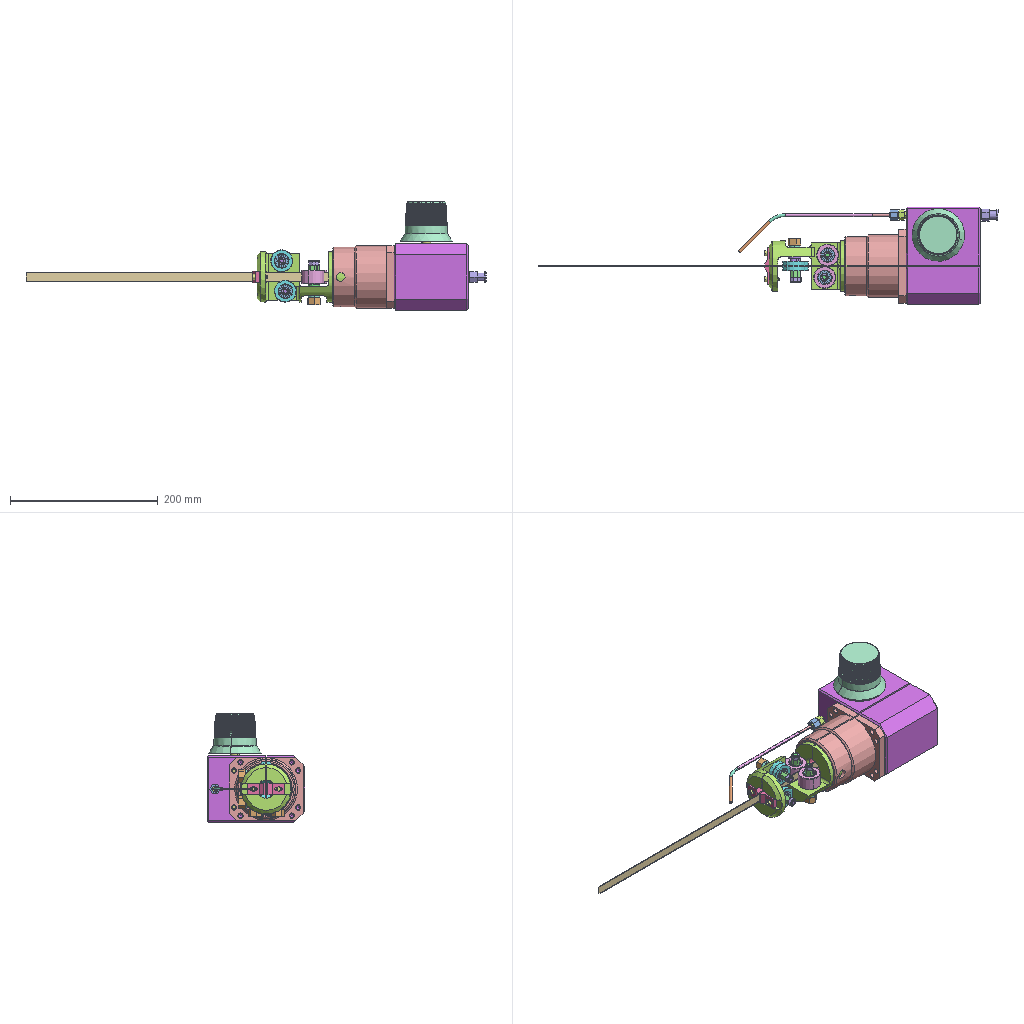Assembly | SolidWorks | 31 different items | 61 placed | box 622 x 132 x 147 mm
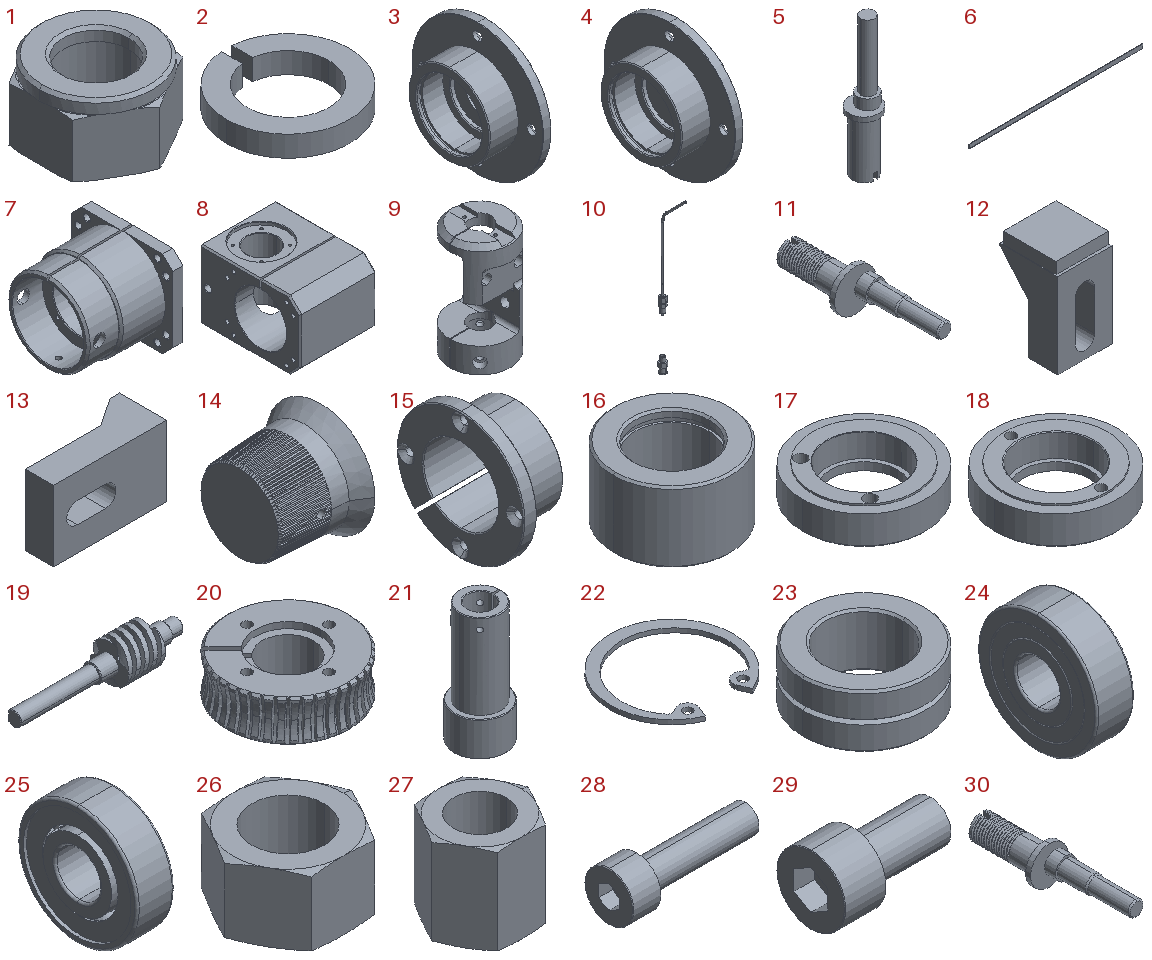Parts list (item | name | quantity | size | volume | features):
1 | - | x4 | 9.8 x 11.05 x 6 mm | 303.009 mm3 | features Cut 3, Boss 1, Chamfer 1, Extrusion 1, MoveFace 1
2 | - | x4 | 15.372 x 15.344 x 2.6 mm | 261.313 mm3 | features Extrusion 1
3 | - | x1 | 18 x 64.5 x 64.5 mm | 18239 mm3 | features CirPattern 2, ICE 2, Chamfer 1, HoleWzd 1, RevCut 1, Revolution 1
4 | - | x1 | 18 x 64.5 x 64.5 mm | 18637 mm3 | features CirPattern 2, Chamfer 1, HoleWzd 1, ICE 1, RevCut 1, Revolution 1
5 | - | x1 | 13 x 13 x 59.5 mm | 3175 mm3 | features ICE 5, Extrusion 1
6 | - | x1 | 503 x 0.6 x 13 mm | 3620 mm3 | features ICE 2, Extrusion 1
7 | - | x1 | 83.2 x 100 x 85 mm | 237929 mm3 | features ICE 5, Chamfer 4, MoveFace 4, MirrorPattern 3, CirPattern 1, DelFace 1, Fillet 1, HoleWzd 1, LockFeature 1, Revolution 1
8 | - | x1 | 100 x 132.3 x 90 mm | 668106 mm3 | features Chamfer 7, ICE 7, HoleWzd 5, DelFace 4, MoveFace 2, CirPattern 1, Extrusion 1, MirrorPattern 1
9 | - | x1 | 67.996 x 68 x 125 mm | 160312 mm3 | features ICE 17, Fillet 8, MoveFace 7, HoleWzd 3, Chamfer 2, DelFace 1, Extrusion 1, MirrorPattern 1
10 | - | x1 | 14 x 58.995 x 350.912 mm | 7220 mm3 | features ICE 8, MoveCopyBody 2, Chamfer 1, MirrorSolid 1, WeldMemberFeat 1, WeldmentFeature 1
11 | - | x2 | 17 x 59.6 x 17 mm | 3396 mm3 | features ICE 5, Chamfer 2, Extrusion 1, SweepThread 1
12 | - | x2 | 14 x 15 x 25 mm | 2645 mm3 | features ICE 4, Extrusion 1
13 | - | x2 | 24 x 10 x 15 mm | 2203 mm3 | features Extrusion 1, ICE 1
14 | - | x1 | 53.8 x 71.2 x 71.2 mm | 101248 mm3 | features Chamfer 1, CirPattern 1, ICE 1, Revolution 1, SweepCut 1
15 | - | x2 | 30 x 68 x 68 mm | 31718 mm3 | features ICE 2, MoveFace 2, Chamfer 1, CirPattern 1, DelFace 1, RevCut 1, Revolution 1
16 | - | x2 | 30 x 30 x 18 mm | 7514 mm3 | features Chamfer 1, Extrusion 1, ICE 1, MirrorPattern 1
17 | - | x1 | 31.5 x 31.5 x 8 mm | 3844 mm3 | features Chamfer 2, ICE 2, Extrusion 1, HoleWzd 1, MirrorPattern 1
18 | - | x1 | 31.5 x 31.5 x 8 mm | 3885 mm3 | features Chamfer 2, ICE 2, Extrusion 1, HoleWzd 1, MirrorPattern 1
19 | - | x1 | 135 x 31.98 x 31.98 mm | 33052 mm3 | features ICE 3, Chamfer 1, CirPattern 1, Helix 1, Revolution 1, SweepCut 1
20 | - | x1 | 60.008 x 60.008 x 20 mm | 38918 mm3 | features ICE 2, CirPattern 1, Helix 1, HoleWzd 1, RefAxis 1, Revolution 1, SweepCut 1
21 | - | x1 | 49.98 x 50 x 118.2 mm | 109781 mm3 | features ICE 6, MoveFace 4, HoleWzd 2, Chamfer 1, CirPattern 1, DelFace 1, Extrusion 1, MirrorPattern 1
22 | - | x2 | 34.4 x 33.091 x 1.2 mm | 292.119 mm3 | features Extrusion 1
23 | - | x2 | 30 x 30 x 13 mm | 5342 mm3 | features DelFace 2, MoveFace 2, Chamfer 1, Extrusion 1, ICE 1, MirrorPattern 1, RevCut 1
24 | - | x8 | 6 x 19 x 19 mm | 1166 mm3 | features Revolution 5, CirPattern 2, RefAxis 1, RevCut 1
25 | - | x2 | 10 x 32 x 32 mm | 4166 mm3 | features Revolution 6, CirPattern 2, RevCut 2, Cut 1, MirrorSolid 1
26 | - | x4 | 17.59 x 15.233 x 9.5 mm | 1159 mm3 | features Cut 2, Chamfer 1, Extrusion 1
27 | - | x4 | 10.89 x 9.431 x 10 mm | 486.676 mm3 | features Cut 2, Chamfer 1, Extrusion 1, MoveFace 1
28 | - | x2 | 20 x 7 x 7 mm | 338.493 mm3 | features BlendCut 1, Cut 1, Fillet 1, LPattern 1, RevCut 1, Revolution 1
29 | - | x2 | 18 x 10 x 10 mm | 743.186 mm3 | features BlendCut 1, Cut 1, Fillet 1, LPattern 1, RevCut 1, Revolution 1
30 | - | x2 | 15 x 59.5 x 15 mm | 3289 mm3 | features ICE 5, Chamfer 2, Extrusion 1, SweepThread 1
31 | GB893.1-86 Holecirclip A Type19 | x1 | - | - | -
Mates (type | each side: item.copy, entity, surface, feature):
Concentric | assembly face | assembly face | 7 times
Coincident | assembly face | assembly face | 9 times
Concentric | 16.1 face cylinder Boss-Extrude1 | assembly face
Coincident | 16.1 face plane Mirror1 | assembly face
Concentric | 16.2 face cylinder Boss-Extrude1 | assembly face
Coincident | 16.2 face plane Cut-Extrude1 | assembly face
Coincident | 16.1 face plane Boss-Extrude1 | 16.2 face plane Boss-Extrude1
Concentric | assembly face | 2.1 face cylinder Extrude1
Coincident | 9.1 face plane Cut-Extrude7 | 2.1 face plane Extrude1
Coincident | 9.1 face plane Cut-Extrude7 | 2.2 face plane Extrude1
Concentric | assembly face | 2.2 face cylinder Extrude1
Concentric | assembly face | 26.1 face cylinder Base-Extrude
Coincident | 2.1 face plane Extrude1 | 26.1 face plane Base-Extrude
Concentric | assembly face | 26.2 face cylinder Base-Extrude
Coincident | 26.1 face plane Base-Extrude | 26.2 face plane Base-Extrude
Concentric | assembly face | 1.1 face cylinder Base-Extrude | 2 times
Coincident | assembly face | 1.1 face plane Base-Extrude
Concentric | assembly face | 1.2 face cylinder Cut-Extrude3
Coincident | assembly face | 1.2 face plane Base-Extrude
Coincident | 17.1 face | 18.1 face
Concentric | 17.1 face | 18.1 face | 2 times
Concentric | 18.1 face | assembly face
Coincident | 18.1 face | assembly face
Concentric | 18.2 face | 17.2 face | 2 times
Coincident | 18.2 face | 17.2 face
Coincident | 18.2 face | assembly face
Coincident | assembly face | 5.1 face
Coincident | assembly face | 5.2 face
Coincident | 17.1 face | 17.2 face
Parallel | 5.1 face | 5.2 face
Concentric | 5.1 face | 2.3 face cylinder Extrude1
Coincident | 9.1 face plane Cut-Extrude4 | 2.3 face plane Extrude1
Concentric | 5.1 face | 26.3 face cylinder Base-Extrude
Coincident | 2.3 face plane Extrude1 | 26.3 face plane Base-Extrude
Concentric | 2.4 face cylinder Extrude1 | 26.4 face cylinder Base-Extrude
Coincident | 2.4 edge | 26.4 face plane Base-Extrude
Coincident | 9.1 face plane Cut-Extrude4 | 2.4 face plane Extrude1
Concentric | 5.2 face | 27.1 face cylinder Base-Extrude
Coincident | assembly face | 27.1 face plane Base-Extrude
Concentric | 5.1 face | 27.2 face cylinder Base-Extrude
Coincident | 27.1 face plane Base-Extrude | 1.3 face plane Base-Extrude
Concentric | 5.2 face | 1.3 face cylinder Cut-Extrude3
Concentric | 5.1 face | 1.4 face cylinder Base-Extrude
Coincident | 27.2 face plane Base-Extrude | 1.4 face plane Base-Extrude
Coincident | 9.1 face plane Cut-Extrude5 | 12.1 face plane Boss-Extrude2
Slot | 12.1 face cylinder Cut-Extrude4 | 9.1 face cylinder M4 Tapped Hole2
Parallel | 9.1 face plane Cut-Extrude5 | 12.1 face plane Cut-Extrude4
Coincident | 9.1 face plane Cut-Extrude5 | 12.2 face plane Boss-Extrude2
Parallel | 9.1 face plane Cut-Extrude5 | 12.2 face plane Boss-Extrude2
Coincident | 9.1 face plane Cut-Extrude2 | 12.2 face plane Boss-Extrude1
Coincident | 9.1 face plane Cut-Extrude2 | 12.1 face plane Boss-Extrude1
Concentric | 9.1 face cylinder Cut-Extrude9 | 21.1 face cylinder Boss-Extrude1
Coincident | 9.1 face plane Cut-Extrude9 | 21.1 face plane Boss-Extrude1
Coincident | 28.1 face plane Base-Revolve | 28.2 face plane Base-Revolve
Coincident | 12.2 face plane Cut-Extrude3 | 28.2 face plane Base-Revolve
Concentric | 9.1 face cylinder M4 Tapped Hole2 | 28.2 face cylinder Base-Revolve
Concentric | 9.1 face cylinder M4 Tapped Hole2 | 28.1 face cylinder Base-Revolve
Concentric | 8.1 face cylinder Cut-Extrude2 | assembly face
Width | assembly face | assembly face | 8.1 face plane Boss-Extrude1 | 8.1 face plane Boss-Extrude1
Concentric | 8.1 face cylinder Cut-Extrude2 | 14.1 face cylinder Revolve1
Concentric | 8.1 face cylinder Cut-Extrude2 | 4.1 face cylinder Revolve1
Coincident | 8.1 face plane Mirror1 | 4.1 face plane Revolve1
Coincident | 4.1 face plane Revolve1 | 22.1 face plane Base-Extrude
Concentric | 8.1 face cylinder Mirror1 | 4.1 face cylinder CirPattern1
Concentric | 8.1 face cylinder Cut-Extrude2 | 3.1 face cylinder Revolve1
Coincident | 3.1 face plane Revolve1 | 22.2 face plane Base-Extrude
Coincident | 8.1 face plane Cut-Extrude6 | 3.1 face plane Revolve1
Concentric | 8.1 face cylinder M4 Tapped Hole1 | 3.1 face cylinder CirPattern1
Concentric | 3.1 face cylinder Cut-Extrude1 | assembly face
Coincident | 14.1 face plane Revolve1 | assembly face
Concentric | 21.1 face cylinder Boss-Extrude1 | assembly face
Coincident | 21.1 face plane Boss-Extrude2 | assembly face
Concentric | 21.1 face cylinder CirPattern1 | assembly face
Slot | 12.2 face cylinder Cut-Extrude4 | 28.2 face cylinder Base-Revolve
Concentric | 22.2 face cylinder Base-Extrude | assembly face
Concentric | 8.1 face cylinder Cut-Extrude2 | 25.1 face cylinder Boss-Revolve4
Concentric | 22.1 face cylinder Base-Extrude | assembly face
Coincident | 25.1 face plane Boss-Revolve4 | assembly face
Concentric | 25.2 face cylinder Boss-Revolve4 | assembly face
Coincident | 25.2 face plane Mirror All1 | assembly face
Concentric | 7.1 face cylinder Revolve1 | 8.1 face cylinder Cut-Extrude1
Parallel | 7.1 face plane Cut-Extrude3 | 8.1 face plane Cut-Extrude5
Coincident | 7.1 face plane Revolve1 | 8.1 face plane Boss-Extrude1
Parallel | 8.1 face plane Boss-Extrude1 | assembly plane
Coincident | 22.2 face plane Base-Extrude | 25.2 face plane Mirror All1
Concentric | 8.1 face cylinder Cut-Extrude1 | 15.1 face cylinder Cut-Extrude2
Coincident | 7.1 face plane Revolve1 | 15.2 face plane Revolve1
Concentric | 7.1 face cylinder CirPattern1 | 15.2 face cylinder CirPattern1
Concentric | 15.1 face cylinder Revolve1 | 15.2 face cylinder Revolve1
Concentric | 15.1 face cylinder Cut-Revolve1 | 15.2 edge
Coincident | 7.1 face plane Revolve1 | 15.1 face plane Revolve1
Concentric | 7.1 face cylinder Revolve1 | 21.1 face cylinder Boss-Extrude2
Parallel | 7.1 face plane Cut-Extrude3 | 9.1 face plane Cut-Extrude2
Coincident | 15.2 face plane Revolve1 | 21.1 face plane Boss-Extrude2
Concentric | assembly face | 23.1 face cylinder Boss-Extrude1
Width | 23.1 face plane Boss-Extrude1 | 23.1 face plane Boss-Extrude1 | assembly face | assembly face
Concentric | 9.1 face cylinder Cut-Extrude12 | assembly face
Coincident | 9.1 face plane Cut-Extrude1 | assembly face
Width | 6.1 face plane Boss-Extrude1 | 6.1 face plane Boss-Extrude1 | 23.1 face plane Cut-Revolve1 | 23.1 face plane Cut-Revolve1
Width | 6.1 face plane Boss-Extrude2 | 6.1 face plane Boss-Extrude2 | 9.1 face plane Cut-Extrude5 | 9.1 face plane Cut-Extrude5
Concentric | assembly face | 23.2 face cylinder Boss-Extrude1
Concentric | 9.1 face cylinder Cut-Extrude12 | 11.1 face cylinder Boss-Extrude2
Coincident | 9.1 face plane Cut-Extrude1 | 11.1 face plane Boss-Extrude1
Concentric | assembly face | 11.1 face cylinder Boss-Extrude4
Coincident | assembly face | 11.1 face plane Boss-Extrude3
Concentric | 27.1 face cylinder Base-Extrude | 11.1 face cylinder Boss-Extrude5
Concentric | 1.3 face cylinder Base-Extrude | 11.1 face cylinder Boss-Extrude5
Concentric | 27.2 face cylinder Base-Extrude | assembly face
Concentric | 1.4 face cylinder Base-Extrude | assembly face
Concentric | 9.1 face cylinder Ø10.5 (10.5) Diameter Hole2 | 30.1 face cylinder Boss-Extrude2
Coincident | 9.1 face plane Cut-Extrude6 | 30.1 face plane Boss-Extrude1
Concentric | 26.1 face cylinder Base-Extrude | 30.1 face cylinder Boss-Extrude2
Concentric | 2.1 face cylinder Extrude1 | 30.1 face cylinder Boss-Extrude1
Concentric | assembly face | 30.1 face cylinder Boss-Extrude4
Coincident | assembly face | 30.1 face plane Boss-Extrude3
Concentric | 1.2 face cylinder Base-Extrude | 30.1 face cylinder Boss-Extrude5
Concentric | 26.2 face cylinder Base-Extrude | 30.2 face cylinder Boss-Extrude2
Coincident | 9.1 face plane Cut-Extrude6 | 30.2 face plane Boss-Extrude1
Concentric | 9.1 face cylinder Ø10.5 (10.5) Diameter Hole2 | 30.2 face cylinder Boss-Extrude2
Concentric | 2.2 face cylinder Extrude1 | 30.2 face cylinder Boss-Extrude1
Concentric | 2.3 face cylinder Extrude1 | assembly edge
Concentric | 2.3 edge | 26.3 face cylinder Base-Extrude
Concentric | 2.4 face cylinder Extrude1 | 11.1 edge
Concentric | 8.1 face cylinder Cut-Extrude11 | 10.1 face cylinder Boss-Extrude6
Width | 10.1 face plane Boss-Extrude1 | 10.1 face plane Cut-Extrude2 | 8.1 face plane Boss-Extrude1 | 8.1 face plane Boss-Extrude1
Parallel | 8.1 face plane Boss-Extrude1 | 10.1 face plane Boss-Extrude5
Coincident | 9.1 face plane Cut-Extrude5 | 13.1 face plane Boss-Extrude1
Slot | 9.1 face cylinder M4 Tapped Hole2 | 13.1 face cylinder Cut-Extrude1
Parallel | 9.1 face plane Cut-Extrude5 | 13.1 face plane Boss-Extrude1
Slot | 13.2 face cylinder Cut-Extrude1 | 9.1 face cylinder M4 Tapped Hole2
Coincident | 9.1 face plane Cut-Extrude5 | 13.2 face plane Boss-Extrude1
Parallel | 9.1 face plane Cut-Extrude5 | 13.2 face plane Boss-Extrude1
Concentric | 21.1 face cylinder Boss-Extrude1 | 20.1 face cylinder Revolve1
Coincident | 21.1 face plane Boss-Extrude2 | 20.1 face plane Revolve1
Coincident | 21.1 face plane Cut-Extrude2 | 20.1 face plane Cut-Extrude2
Concentric | 25.1 face cylinder Boss-Revolve4 | 19.1 face cylinder Revolve1
Coincident | 25.1 face plane Boss-Revolve4 | 19.1 face plane Revolve1
Concentric | 9.1 face cylinder Cut-Extrude12 | 11.2 face cylinder Boss-Extrude1
Coincident | 9.1 face plane Cut-Extrude1 | 11.2 face plane Boss-Extrude1
Concentric | assembly face | 11.2 face cylinder Boss-Extrude3
Coincident | assembly face | 11.2 face plane Boss-Extrude3
Concentric | 27.2 face cylinder Base-Extrude | 11.2 face cylinder Boss-Extrude5
Concentric | 1.4 face cylinder Base-Extrude | 11.2 face cylinder Boss-Extrude5
Coincident | 25.2 face plane Mirror All1 | 19.1 face plane Revolve1
Concentric | 26.3 face cylinder Base-Extrude | 11.2 face cylinder Boss-Extrude1
Concentric | 14.1 face cylinder Revolve1 | 19.1 face cylinder Revolve1
Coincident | 14.1 face plane Revolve1 | 19.1 face plane Cut-Extrude2
Concentric | 30.1 face cylinder Boss-Extrude4 | 24.1 face cylinder Revolve1
Coincident | 30.1 face plane Boss-Extrude3 | 24.1 face plane Revolve1
Concentric | 30.1 face cylinder Boss-Extrude4 | 24.2 face cylinder Revolve1
Coincident | 24.1 face plane Revolve1 | 24.2 face plane Revolve1
Concentric | 30.2 face cylinder Boss-Extrude4 | 24.3 face cylinder Revolve1
Coincident | 30.2 face plane Boss-Extrude3 | 24.3 face plane Revolve1
Concentric | 30.2 face cylinder Boss-Extrude4 | 24.4 face cylinder Revolve1
Coincident | 24.3 face plane Revolve1 | 24.4 face plane Revolve1
Concentric | 1.1 face cylinder Base-Extrude | 30.2 face cylinder Boss-Extrude5
Concentric | 11.1 face cylinder Boss-Extrude4 | 24.5 face cylinder Revolve1
Coincident | 11.1 face plane Boss-Extrude3 | 24.5 face plane Revolve1
Concentric | 11.1 face cylinder Boss-Extrude4 | 24.6 face cylinder Revolve1
Coincident | 24.5 face plane Revolve1 | 24.6 face plane Revolve1
Concentric | 23.1 face cylinder Boss-Extrude1 | 24.5 face cylinder Revolve1
Width | 23.1 face plane Boss-Extrude1 | 23.1 face plane Boss-Extrude1 | 24.5 face plane Revolve1 | 24.6 face plane Revolve1
Concentric | 11.2 face cylinder Boss-Extrude4 | 24.7 face cylinder Revolve1
Coincident | 11.2 face plane Boss-Extrude3 | 24.7 face plane Revolve1
Concentric | 11.2 face cylinder Boss-Extrude4 | 24.8 face cylinder Revolve1
Coincident | 24.7 face plane Revolve1 | 24.8 face plane Revolve1
Concentric | 23.2 face cylinder Boss-Extrude1 | 24.7 face cylinder Revolve1
Width | 23.2 face plane Boss-Extrude1 | 23.2 face plane Boss-Extrude1 | 24.8 face plane Revolve1 | 24.7 face plane Revolve1
Coincident | 27.2 face plane Base-Extrude | 24.8 face plane Revolve1
Coincident | 27.1 face plane Base-Extrude | 24.6 face plane Revolve1
Concentric | 30.1 face cylinder Boss-Extrude5 | 27.3 face cylinder Base-Extrude
Coincident | 24.2 face plane Revolve1 | 27.3 face plane Base-Extrude
Coincident | 1.2 face plane Base-Extrude | 27.3 face plane Base-Extrude
Concentric | 30.2 face cylinder Boss-Extrude5 | 27.4 face cylinder Base-Extrude
Coincident | 24.4 face plane Revolve1 | 27.4 face plane Base-Extrude
Coincident | 1.1 face plane Base-Extrude | 27.4 face plane Base-Extrude
Concentric | 25.2 face cylinder Boss-Revolve4 | 19.1 face cylinder Revolve1
Concentric | 22.2 face cylinder Base-Extrude | 19.1 face cylinder Revolve1
Concentric | 22.1 face cylinder Base-Extrude | 19.1 face cylinder Revolve1
Concentric | 21.1 face cylinder Cut-Extrude7 | 29.1 face cylinder Base-Revolve
Concentric | 21.1 face cylinder Cut-Extrude7 | 29.2 face cylinder Base-Revolve
Coincident | 9.1 face plane Cut-Extrude16 | 29.1 face plane Base-Revolve
Coincident | 9.1 face plane Cut-Extrude15 | 29.2 face plane Base-Revolve